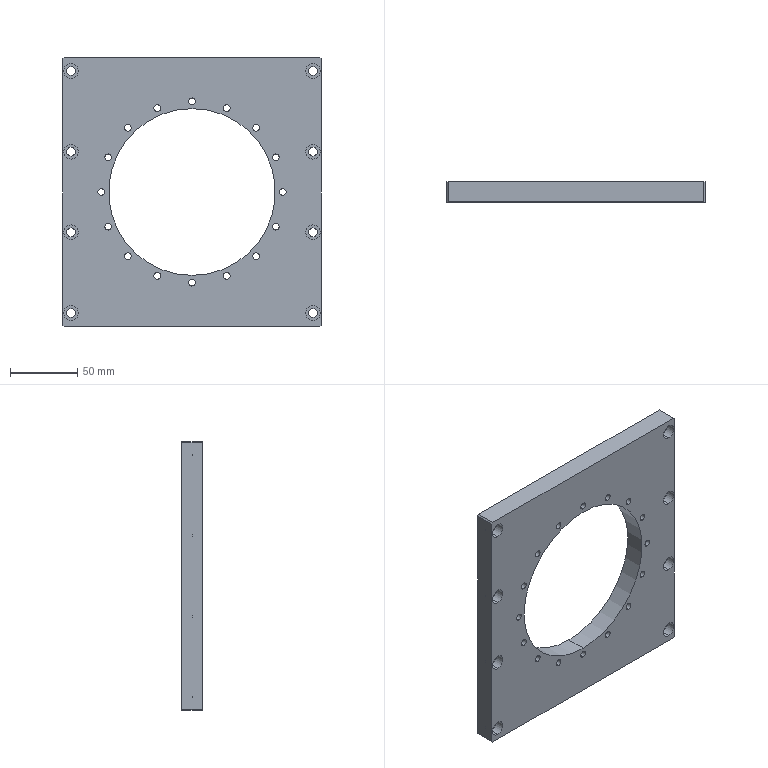Part | SolidWorks | features HoleWzd 2, Chamfer 1, Extrusion 1, ICE 1 | 1 solid | 84 faces | box 192 x 15 x 200 mm | volume 382699 mm3 | cylinder 66 | plane 18 | commonest cylinder face diameters 5 x32 6.6 x16 11 x16 124 x2